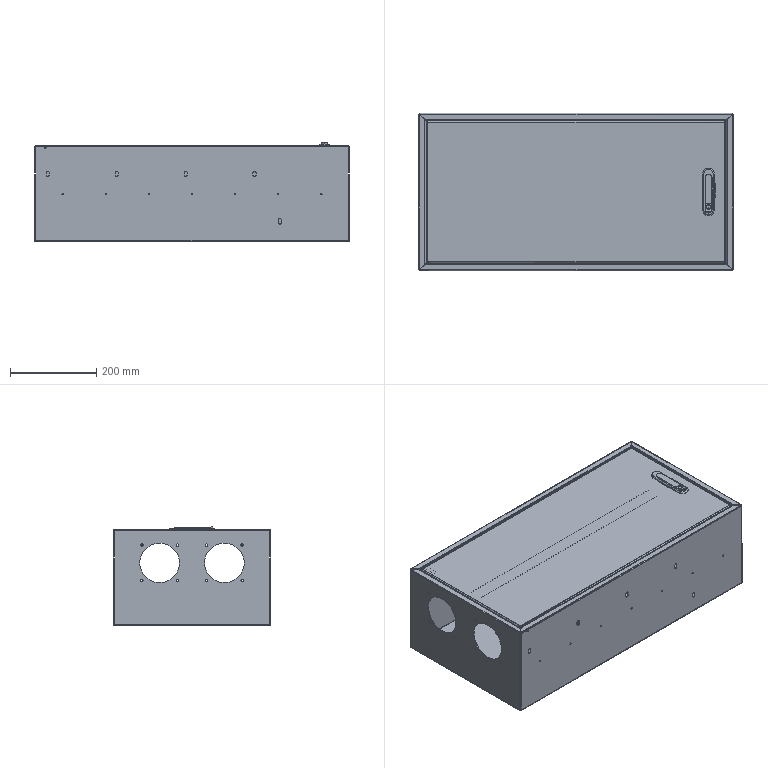Part | SolidWorks | 12 solids | 804 faces | box 730 x 365 x 229.027 mm | volume 2279272 mm3 | cylinder 358 | plane 357 | spline 58 | cone 25 | torus 6 | commonest cylinder face diameters 3.3 x142 5.5 x32 1.473 x30 7 x19 4 x18 4.473 x18